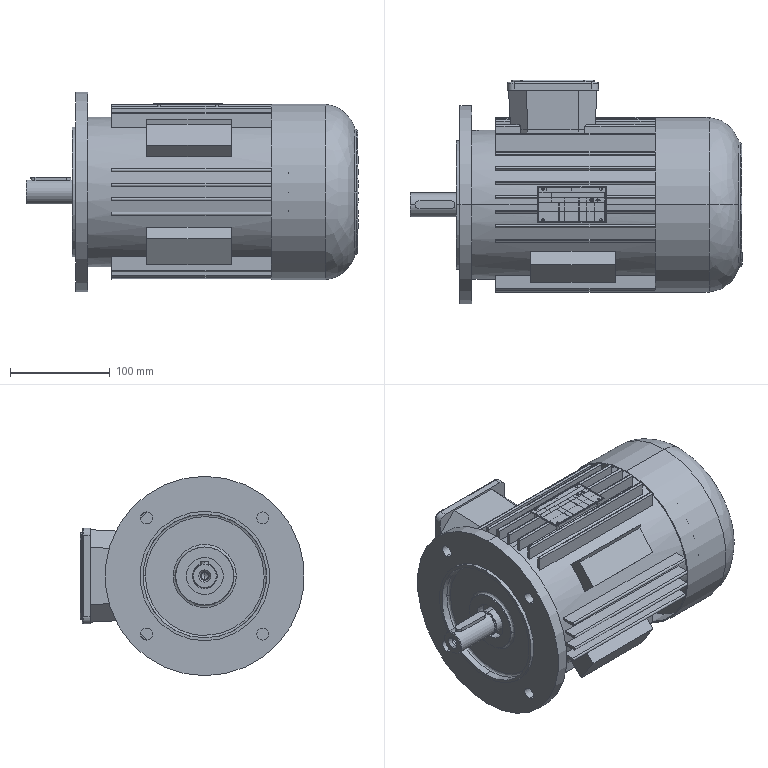Part | SolidWorks | features ICE 3, BaseBody 1 | 1 solid | 494 faces | box 333 x 225 x 200 mm | volume 6079117 mm3 | plane 319 | cylinder 127 | spline 20 | cone 20 | torus 8 | commonest cylinder face diameters 3 x51 2 x8 4 x8 12 x8 8 x5 2.5 x4